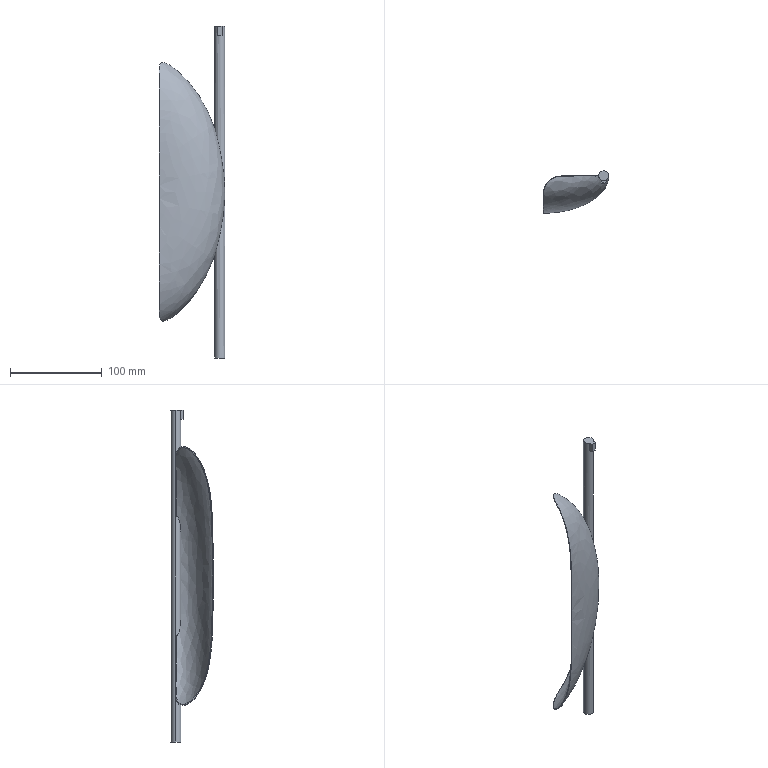Part | SolidWorks | features ICE 4, Attribute 3, Cut 3, Chamfer 2, ExtruThin 1, Fillet 1, Shell 1, Sweep 1 | 1 solid | 31 faces | box 71.359 x 45.899 x 361 mm | volume 54038 mm3 | plane 15 | spline 10 | cylinder 6 | commonest cylinder face diameters 11 x4 40 x2